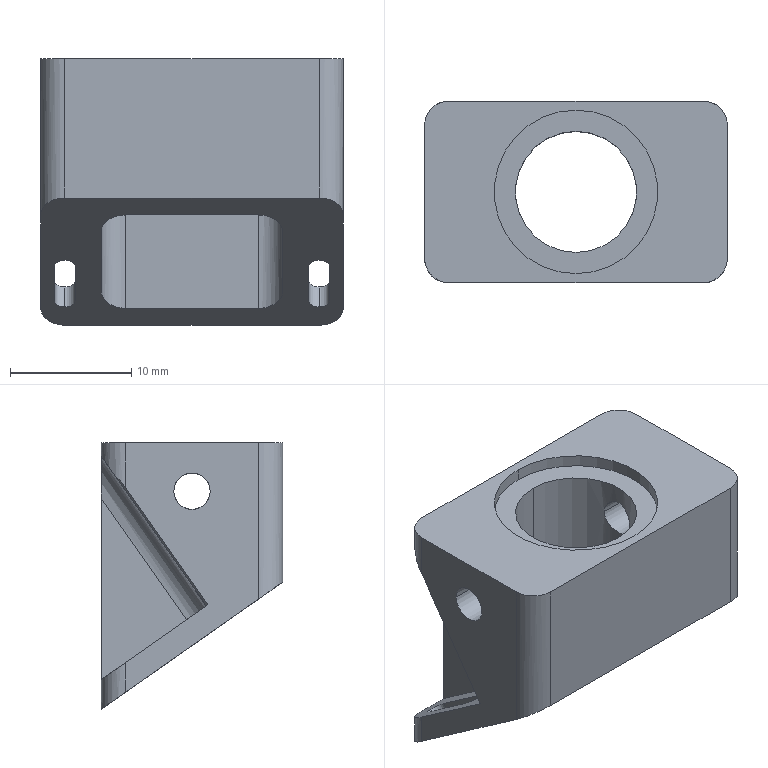Part | 1 solid | 62 faces | box 25 x 15 x 22 mm | volume 3583 mm3 | cylinder 34 | plane 28 | commonest cylinder face diameters 4 x12 1.6 x8 1.7 x6 3 x4 10 x2 13.5 x2